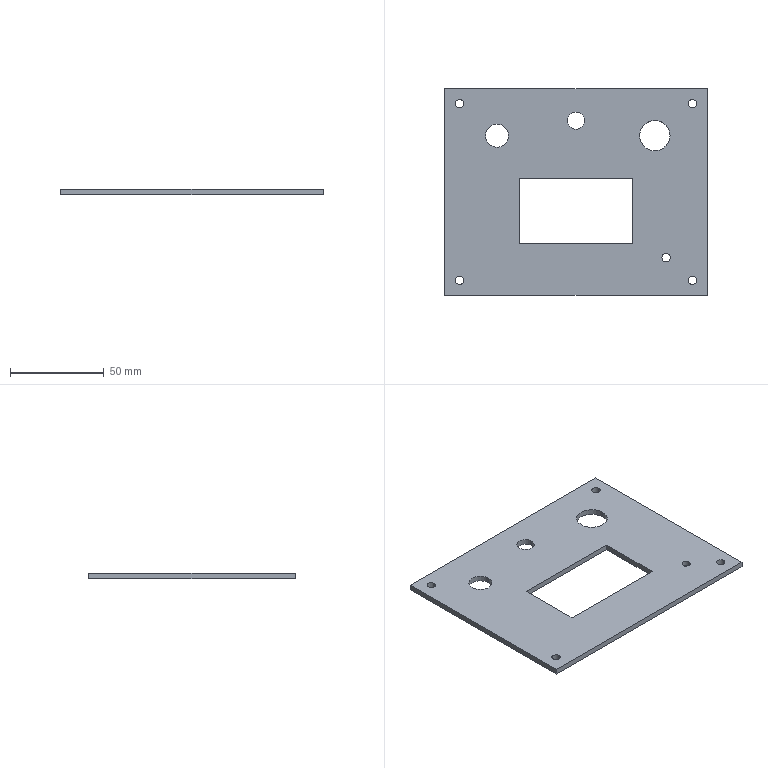Part | SolidWorks | features Extrusion 1 | 1 solid | 26 faces | box 140 x 110 x 3 mm | volume 38560 mm3 | cylinder 16 | plane 10 | commonest cylinder face diameters 4.5 x10 9.2 x2 12.2 x2 16.2 x2
STEP:
#1=CARTESIAN_POINT('',(45.75,-35.,-1.5));
#2=VERTEX_POINT('',#1);
#3=CARTESIAN_POINT('',(50.25,-35.,-1.5));
#4=VERTEX_POINT('',#3);
#5=CARTESIAN_POINT('',(48.,-35.,-1.5));
#6=DIRECTION('',(0.,0.,1.));
#7=DIRECTION('',(1.,0.,0.));
#8=AXIS2_PLACEMENT_3D('',#5,#6,#7);
#9=CIRCLE('',#8,2.25);
#10=EDGE_CURVE('',#2,#4,#9,.T.);
#11=ORIENTED_EDGE('',*,*,#10,.F.);
#12=CARTESIAN_POINT('',(45.75,-35.,1.5));
#13=VERTEX_POINT('',#12);
#14=CARTESIAN_POINT('',(45.75,-35.,-1.5));
#15=DIRECTION('',(0.,0.,1.));
#16=VECTOR('',#15,1000.);
#17=LINE('',#14,#16);
#18=EDGE_CURVE('',#2,#13,#17,.T.);
#19=ORIENTED_EDGE('',*,*,#18,.T.);
#20=CARTESIAN_POINT('',(50.25,-35.,1.5));
#21=VERTEX_POINT('',#20);
#22=CARTESIAN_POINT('',(48.,-35.,1.5));
#23=DIRECTION('',(0.,0.,1.));
#24=DIRECTION('',(1.,0.,0.));
#25=AXIS2_PLACEMENT_3D('',#22,#23,#24);
#26=CIRCLE('',#25,2.25);
#27=EDGE_CURVE('',#13,#21,#26,.T.);
#28=ORIENTED_EDGE('',*,*,#27,.T.);
#29=CARTESIAN_POINT('',(50.25,-35.,-1.5));
#30=DIRECTION('',(0.,0.,1.));
#31=VECTOR('',#30,1000.);
#32=LINE('',#29,#31);
#33=EDGE_CURVE('',#4,#21,#32,.T.);
#34=ORIENTED_EDGE('',*,*,#33,.F.);
#35=EDGE_LOOP('',(#11,#19,#28,#34));
#36=FACE_OUTER_BOUND('',#35,.T.);
#37=CARTESIAN_POINT('',(48.,-35.,-1.5));
#38=DIRECTION('',(0.,0.,1.));
#39=DIRECTION('',(1.,0.,0.));
#40=AXIS2_PLACEMENT_3D('',#37,#38,#39);
#41=CYLINDRICAL_SURFACE('',#40,2.25);
#42=ADVANCED_FACE('',(#36),#41,.F.);
#43=CARTESIAN_POINT('',(-4.6,38.,-1.5));
#44=VERTEX_POINT('',#43);
#45=CARTESIAN_POINT('',(4.6,38.,-1.5));
#46=VERTEX_POINT('',#45);
#47=CARTESIAN_POINT('',(0.,38.,-1.5));
#48=DIRECTION('',(0.,0.,1.));
#49=DIRECTION('',(1.,0.,0.));
#50=AXIS2_PLACEMENT_3D('',#47,#48,#49);
#51=CIRCLE('',#50,4.6);
#52=EDGE_CURVE('',#44,#46,#51,.T.);
#53=ORIENTED_EDGE('',*,*,#52,.F.);
#54=CARTESIAN_POINT('',(-4.6,38.,1.5));
#55=VERTEX_POINT('',#54);
#56=CARTESIAN_POINT('',(-4.6,38.,-1.5));
#57=DIRECTION('',(0.,0.,1.));
#58=VECTOR('',#57,1000.);
#59=LINE('',#56,#58);
#60=EDGE_CURVE('',#44,#55,#59,.T.);
#61=ORIENTED_EDGE('',*,*,#60,.T.);
#62=CARTESIAN_POINT('',(4.6,38.,1.5));
#63=VERTEX_POINT('',#62);
#64=CARTESIAN_POINT('',(0.,38.,1.5));
#65=DIRECTION('',(0.,0.,1.));
#66=DIRECTION('',(1.,0.,0.));
#67=AXIS2_PLACEMENT_3D('',#64,#65,#66);
#68=CIRCLE('',#67,4.6);
#69=EDGE_CURVE('',#55,#63,#68,.T.);
#70=ORIENTED_EDGE('',*,*,#69,.T.);
#71=CARTESIAN_POINT('',(4.6,38.,-1.5));
#72=DIRECTION('',(0.,0.,1.));
#73=VECTOR('',#72,1000.);
#74=LINE('',#71,#73);
#75=EDGE_CURVE('',#46,#63,#74,.T.);
#76=ORIENTED_EDGE('',*,*,#75,.F.);
#77=EDGE_LOOP('',(#53,#61,#70,#76));
#78=FACE_OUTER_BOUND('',#77,.T.);
#79=CARTESIAN_POINT('',(0.,38.,-1.5));
#80=DIRECTION('',(0.,0.,1.));
#81=DIRECTION('',(1.,0.,0.));
#82=AXIS2_PLACEMENT_3D('',#79,#80,#81);
#83=CYLINDRICAL_SURFACE('',#82,4.6);
#84=ADVANCED_FACE('',(#78),#83,.F.);
#85=CARTESIAN_POINT('',(33.9,30.,-1.5));
#86=VERTEX_POINT('',#85);
#87=CARTESIAN_POINT('',(50.1,30.,-1.5));
#88=VERTEX_POINT('',#87);
#89=CARTESIAN_POINT('',(42.,30.,-1.5));
#90=DIRECTION('',(0.,0.,1.));
#91=DIRECTION('',(1.,0.,0.));
#92=AXIS2_PLACEMENT_3D('',#89,#90,#91);
#93=CIRCLE('',#92,8.1);
#94=EDGE_CURVE('',#86,#88,#93,.T.);
#95=ORIENTED_EDGE('',*,*,#94,.F.);
#96=CARTESIAN_POINT('',(33.9,30.,1.5));
#97=VERTEX_POINT('',#96);
#98=CARTESIAN_POINT('',(33.9,30.,-1.5));
#99=DIRECTION('',(0.,0.,1.));
#100=VECTOR('',#99,1000.);
#101=LINE('',#98,#100);
#102=EDGE_CURVE('',#86,#97,#101,.T.);
#103=ORIENTED_EDGE('',*,*,#102,.T.);
#104=CARTESIAN_POINT('',(50.1,30.,1.5));
#105=VERTEX_POINT('',#104);
#106=CARTESIAN_POINT('',(42.,30.,1.5));
#107=DIRECTION('',(0.,0.,1.));
#108=DIRECTION('',(1.,0.,0.));
#109=AXIS2_PLACEMENT_3D('',#106,#107,#108);
#110=CIRCLE('',#109,8.1);
#111=EDGE_CURVE('',#97,#105,#110,.T.);
#112=ORIENTED_EDGE('',*,*,#111,.T.);
#113=CARTESIAN_POINT('',(50.1,30.,-1.5));
#114=DIRECTION('',(0.,0.,1.));
#115=VECTOR('',#114,1000.);
#116=LINE('',#113,#115);
#117=EDGE_CURVE('',#88,#105,#116,.T.);
#118=ORIENTED_EDGE('',*,*,#117,.F.);
#119=EDGE_LOOP('',(#95,#103,#112,#118));
#120=FACE_OUTER_BOUND('',#119,.T.);
#121=CARTESIAN_POINT('',(42.,30.,-1.5));
#122=DIRECTION('',(0.,0.,1.));
#123=DIRECTION('',(1.,0.,0.));
#124=AXIS2_PLACEMENT_3D('',#121,#122,#123);
#125=CYLINDRICAL_SURFACE('',#124,8.1);
#126=ADVANCED_FACE('',(#120),#125,.F.);
#127=CARTESIAN_POINT('',(-48.1,30.,-1.5));
#128=VERTEX_POINT('',#127);
#129=CARTESIAN_POINT('',(-35.9,30.,-1.5));
#130=VERTEX_POINT('',#129);
#131=CARTESIAN_POINT('',(-42.,30.,-1.5));
#132=DIRECTION('',(0.,0.,1.));
#133=DIRECTION('',(1.,0.,0.));
#134=AXIS2_PLACEMENT_3D('',#131,#132,#133);
#135=CIRCLE('',#134,6.1);
#136=EDGE_CURVE('',#128,#130,#135,.T.);
#137=ORIENTED_EDGE('',*,*,#136,.F.);
#138=CARTESIAN_POINT('',(-48.1,30.,1.5));
#139=VERTEX_POINT('',#138);
#140=CARTESIAN_POINT('',(-48.1,30.,-1.5));
#141=DIRECTION('',(0.,0.,1.));
#142=VECTOR('',#141,1000.);
#143=LINE('',#140,#142);
#144=EDGE_CURVE('',#128,#139,#143,.T.);
#145=ORIENTED_EDGE('',*,*,#144,.T.);
#146=CARTESIAN_POINT('',(-35.9,30.,1.5));
#147=VERTEX_POINT('',#146);
#148=CARTESIAN_POINT('',(-42.,30.,1.5));
#149=DIRECTION('',(0.,0.,1.));
#150=DIRECTION('',(1.,0.,0.));
#151=AXIS2_PLACEMENT_3D('',#148,#149,#150);
#152=CIRCLE('',#151,6.1);
#153=EDGE_CURVE('',#139,#147,#152,.T.);
#154=ORIENTED_EDGE('',*,*,#153,.T.);
#155=CARTESIAN_POINT('',(-35.9,30.,-1.5));
#156=DIRECTION('',(0.,0.,1.));
#157=VECTOR('',#156,1000.);
#158=LINE('',#155,#157);
#159=EDGE_CURVE('',#130,#147,#158,.T.);
#160=ORIENTED_EDGE('',*,*,#159,.F.);
#161=EDGE_LOOP('',(#137,#145,#154,#160));
#162=FACE_OUTER_BOUND('',#161,.T.);
#163=CARTESIAN_POINT('',(-42.,30.,-1.5));
#164=DIRECTION('',(0.,0.,1.));
#165=DIRECTION('',(1.,0.,0.));
#166=AXIS2_PLACEMENT_3D('',#163,#164,#165);
#167=CYLINDRICAL_SURFACE('',#166,6.1);
#168=ADVANCED_FACE('',(#162),#167,.F.);
#169=CARTESIAN_POINT('',(59.75,47.,-1.5));
#170=VERTEX_POINT('',#169);
#171=CARTESIAN_POINT('',(64.25,47.,-1.5));
#172=VERTEX_POINT('',#171);
#173=CARTESIAN_POINT('',(62.,47.,-1.5));
#174=DIRECTION('',(0.,0.,1.));
#175=DIRECTION('',(1.,0.,0.));
#176=AXIS2_PLACEMENT_3D('',#173,#174,#175);
#177=CIRCLE('',#176,2.25);
#178=EDGE_CURVE('',#170,#172,#177,.T.);
#179=ORIENTED_EDGE('',*,*,#178,.F.);
#180=CARTESIAN_POINT('',(59.75,47.,1.5));
#181=VERTEX_POINT('',#180);
#182=CARTESIAN_POINT('',(59.75,47.,-1.5));
#183=DIRECTION('',(0.,0.,1.));
#184=VECTOR('',#183,1000.);
#185=LINE('',#182,#184);
#186=EDGE_CURVE('',#170,#181,#185,.T.);
#187=ORIENTED_EDGE('',*,*,#186,.T.);
#188=CARTESIAN_POINT('',(64.25,47.,1.5));
#189=VERTEX_POINT('',#188);
#190=CARTESIAN_POINT('',(62.,47.,1.5));
#191=DIRECTION('',(0.,0.,1.));
#192=DIRECTION('',(1.,0.,0.));
#193=AXIS2_PLACEMENT_3D('',#190,#191,#192);
#194=CIRCLE('',#193,2.25);
#195=EDGE_CURVE('',#181,#189,#194,.T.);
#196=ORIENTED_EDGE('',*,*,#195,.T.);
#197=CARTESIAN_POINT('',(64.25,47.,-1.5));
#198=DIRECTION('',(0.,0.,1.));
#199=VECTOR('',#198,1000.);
#200=LINE('',#197,#199);
#201=EDGE_CURVE('',#172,#189,#200,.T.);
#202=ORIENTED_EDGE('',*,*,#201,.F.);
#203=EDGE_LOOP('',(#179,#187,#196,#202));
#204=FACE_OUTER_BOUND('',#203,.T.);
#205=CARTESIAN_POINT('',(62.,47.,-1.5));
#206=DIRECTION('',(0.,0.,1.));
#207=DIRECTION('',(1.,0.,0.));
#208=AXIS2_PLACEMENT_3D('',#205,#206,#207);
#209=CYLINDRICAL_SURFACE('',#208,2.25);
#210=ADVANCED_FACE('',(#204),#209,.F.);
#211=CARTESIAN_POINT('',(59.75,-47.,-1.5));
#212=VERTEX_POINT('',#211);
#213=CARTESIAN_POINT('',(64.25,-47.,-1.5));
#214=VERTEX_POINT('',#213);
#215=CARTESIAN_POINT('',(62.,-47.,-1.5));
#216=DIRECTION('',(0.,0.,1.));
#217=DIRECTION('',(1.,0.,0.));
#218=AXIS2_PLACEMENT_3D('',#215,#216,#217);
#219=CIRCLE('',#218,2.25);
#220=EDGE_CURVE('',#212,#214,#219,.T.);
#221=ORIENTED_EDGE('',*,*,#220,.F.);
#222=CARTESIAN_POINT('',(59.75,-47.,1.5));
#223=VERTEX_POINT('',#222);
#224=CARTESIAN_POINT('',(59.75,-47.,-1.5));
#225=DIRECTION('',(0.,0.,1.));
#226=VECTOR('',#225,1000.);
#227=LINE('',#224,#226);
#228=EDGE_CURVE('',#212,#223,#227,.T.);
#229=ORIENTED_EDGE('',*,*,#228,.T.);
#230=CARTESIAN_POINT('',(64.25,-47.,1.5));
#231=VERTEX_POINT('',#230);
#232=CARTESIAN_POINT('',(62.,-47.,1.5));
#233=DIRECTION('',(0.,0.,1.));
#234=DIRECTION('',(1.,0.,0.));
#235=AXIS2_PLACEMENT_3D('',#232,#233,#234);
#236=CIRCLE('',#235,2.25);
#237=EDGE_CURVE('',#223,#231,#236,.T.);
#238=ORIENTED_EDGE('',*,*,#237,.T.);
#239=CARTESIAN_POINT('',(64.25,-47.,-1.5));
#240=DIRECTION('',(0.,0.,1.));
#241=VECTOR('',#240,1000.);
#242=LINE('',#239,#241);
#243=EDGE_CURVE('',#214,#231,#242,.T.);
#244=ORIENTED_EDGE('',*,*,#243,.F.);
#245=EDGE_LOOP('',(#221,#229,#238,#244));
#246=FACE_OUTER_BOUND('',#245,.T.);
#247=CARTESIAN_POINT('',(62.,-47.,-1.5));
#248=DIRECTION('',(0.,0.,1.));
#249=DIRECTION('',(1.,0.,0.));
#250=AXIS2_PLACEMENT_3D('',#247,#248,#249);
#251=CYLINDRICAL_SURFACE('',#250,2.25);
#252=ADVANCED_FACE('',(#246),#251,.F.);
#253=CARTESIAN_POINT('',(-64.25,47.,-1.5));
#254=VERTEX_POINT('',#253);
#255=CARTESIAN_POINT('',(-59.75,47.,-1.5));
#256=VERTEX_POINT('',#255);
#257=CARTESIAN_POINT('',(-62.,47.,-1.5));
#258=DIRECTION('',(0.,0.,1.));
#259=DIRECTION('',(1.,0.,0.));
#260=AXIS2_PLACEMENT_3D('',#257,#258,#259);
#261=CIRCLE('',#260,2.25);
#262=EDGE_CURVE('',#254,#256,#261,.T.);
#263=ORIENTED_EDGE('',*,*,#262,.F.);
#264=CARTESIAN_POINT('',(-64.25,47.,1.5));
#265=VERTEX_POINT('',#264);
#266=CARTESIAN_POINT('',(-64.25,47.,-1.5));
#267=DIRECTION('',(0.,0.,1.));
#268=VECTOR('',#267,1000.);
#269=LINE('',#266,#268);
#270=EDGE_CURVE('',#254,#265,#269,.T.);
#271=ORIENTED_EDGE('',*,*,#270,.T.);
#272=CARTESIAN_POINT('',(-59.75,47.,1.5));
#273=VERTEX_POINT('',#272);
#274=CARTESIAN_POINT('',(-62.,47.,1.5));
#275=DIRECTION('',(0.,0.,1.));
#276=DIRECTION('',(1.,0.,0.));
#277=AXIS2_PLACEMENT_3D('',#274,#275,#276);
#278=CIRCLE('',#277,2.25);
#279=EDGE_CURVE('',#265,#273,#278,.T.);
#280=ORIENTED_EDGE('',*,*,#279,.T.);
#281=CARTESIAN_POINT('',(-59.75,47.,-1.5));
#282=DIRECTION('',(0.,0.,1.));
#283=VECTOR('',#282,1000.);
#284=LINE('',#281,#283);
#285=EDGE_CURVE('',#256,#273,#284,.T.);
#286=ORIENTED_EDGE('',*,*,#285,.F.);
#287=EDGE_LOOP('',(#263,#271,#280,#286));
#288=FACE_OUTER_BOUND('',#287,.T.);
#289=CARTESIAN_POINT('',(-62.,47.,-1.5));
#290=DIRECTION('',(0.,0.,1.));
#291=DIRECTION('',(1.,0.,0.));
#292=AXIS2_PLACEMENT_3D('',#289,#290,#291);
#293=CYLINDRICAL_SURFACE('',#292,2.25);
#294=ADVANCED_FACE('',(#288),#293,.F.);
#295=CARTESIAN_POINT('',(-64.25,-47.,-1.5));
#296=VERTEX_POINT('',#295);
#297=CARTESIAN_POINT('',(-59.75,-47.,-1.5));
#298=VERTEX_POINT('',#297);
#299=CARTESIAN_POINT('',(-62.,-47.,-1.5));
#300=DIRECTION('',(0.,0.,1.));
#301=DIRECTION('',(1.,0.,0.));
#302=AXIS2_PLACEMENT_3D('',#299,#300,#301);
#303=CIRCLE('',#302,2.25);
#304=EDGE_CURVE('',#296,#298,#303,.T.);
#305=ORIENTED_EDGE('',*,*,#304,.F.);
#306=CARTESIAN_POINT('',(-64.25,-47.,1.5));
#307=VERTEX_POINT('',#306);
#308=CARTESIAN_POINT('',(-64.25,-47.,-1.5));
#309=DIRECTION('',(0.,0.,1.));
#310=VECTOR('',#309,1000.);
#311=LINE('',#308,#310);
#312=EDGE_CURVE('',#296,#307,#311,.T.);
#313=ORIENTED_EDGE('',*,*,#312,.T.);
#314=CARTESIAN_POINT('',(-59.75,-47.,1.5));
#315=VERTEX_POINT('',#314);
#316=CARTESIAN_POINT('',(-62.,-47.,1.5));
#317=DIRECTION('',(0.,0.,1.));
#318=DIRECTION('',(1.,0.,0.));
#319=AXIS2_PLACEMENT_3D('',#316,#317,#318);
#320=CIRCLE('',#319,2.25);
#321=EDGE_CURVE('',#307,#315,#320,.T.);
#322=ORIENTED_EDGE('',*,*,#321,.T.);
#323=CARTESIAN_POINT('',(-59.75,-47.,-1.5));
#324=DIRECTION('',(0.,0.,1.));
#325=VECTOR('',#324,1000.);
#326=LINE('',#323,#325);
#327=EDGE_CURVE('',#298,#315,#326,.T.);
#328=ORIENTED_EDGE('',*,*,#327,.F.);
#329=EDGE_LOOP('',(#305,#313,#322,#328));
#330=FACE_OUTER_BOUND('',#329,.T.);
#331=CARTESIAN_POINT('',(-62.,-47.,-1.5));
#332=DIRECTION('',(0.,0.,1.));
#333=DIRECTION('',(1.,0.,0.));
#334=AXIS2_PLACEMENT_3D('',#331,#332,#333);
#335=CYLINDRICAL_SURFACE('',#334,2.25);
#336=ADVANCED_FACE('',(#330),#335,.F.);
#337=CARTESIAN_POINT('',(-70.,55.,1.5));
#338=VERTEX_POINT('',#337);
#339=CARTESIAN_POINT('',(-70.,-55.,1.5));
#340=VERTEX_POINT('',#339);
#341=CARTESIAN_POINT('',(-70.,55.,1.5));
#342=DIRECTION('',(0.,-1.,0.));
#343=VECTOR('',#342,1000.);
#344=LINE('',#341,#343);
#345=EDGE_CURVE('',#338,#340,#344,.T.);
#346=ORIENTED_EDGE('',*,*,#345,.F.);
#347=CARTESIAN_POINT('',(-70.,55.,-1.5));
#348=VERTEX_POINT('',#347);
#349=CARTESIAN_POINT('',(-70.,55.,-1.5));
#350=DIRECTION('',(0.,0.,1.));
#351=VECTOR('',#350,1000.);
#352=LINE('',#349,#351);
#353=EDGE_CURVE('',#348,#338,#352,.T.);
#354=ORIENTED_EDGE('',*,*,#353,.F.);
#355=CARTESIAN_POINT('',(-70.,-55.,-1.5));
#356=VERTEX_POINT('',#355);
#357=CARTESIAN_POINT('',(-70.,55.,-1.5));
#358=DIRECTION('',(0.,-1.,0.));
#359=VECTOR('',#358,1000.);
#360=LINE('',#357,#359);
#361=EDGE_CURVE('',#348,#356,#360,.T.);
#362=ORIENTED_EDGE('',*,*,#361,.T.);
#363=CARTESIAN_POINT('',(-70.,-55.,-1.5));
#364=DIRECTION('',(0.,0.,1.));
#365=VECTOR('',#364,1000.);
#366=LINE('',#363,#365);
#367=EDGE_CURVE('',#356,#340,#366,.T.);
#368=ORIENTED_EDGE('',*,*,#367,.T.);
#369=EDGE_LOOP('',(#346,#354,#362,#368));
#370=FACE_OUTER_BOUND('',#369,.T.);
#371=CARTESIAN_POINT('',(-70.,55.,-1.5));
#372=DIRECTION('',(-1.,0.,0.));
#373=DIRECTION('',(0.,0.,1.));
#374=AXIS2_PLACEMENT_3D('',#371,#372,#373);
#375=PLANE('',#374);
#376=ADVANCED_FACE('',(#370),#375,.T.);
#377=CARTESIAN_POINT('',(70.,55.,1.5));
#378=VERTEX_POINT('',#377);
#379=CARTESIAN_POINT('',(70.,55.,1.5));
#380=DIRECTION('',(-1.,0.,0.));
#381=VECTOR('',#380,1000.);
#382=LINE('',#379,#381);
#383=EDGE_CURVE('',#378,#338,#382,.T.);
#384=ORIENTED_EDGE('',*,*,#383,.F.);
#385=CARTESIAN_POINT('',(70.,55.,-1.5));
#386=VERTEX_POINT('',#385);
#387=CARTESIAN_POINT('',(70.,55.,-1.5));
#388=DIRECTION('',(0.,0.,1.));
#389=VECTOR('',#388,1000.);
#390=LINE('',#387,#389);
#391=EDGE_CURVE('',#386,#378,#390,.T.);
#392=ORIENTED_EDGE('',*,*,#391,.F.);
#393=CARTESIAN_POINT('',(70.,55.,-1.5));
#394=DIRECTION('',(-1.,0.,0.));
#395=VECTOR('',#394,1000.);
#396=LINE('',#393,#395);
#397=EDGE_CURVE('',#386,#348,#396,.T.);
#398=ORIENTED_EDGE('',*,*,#397,.T.);
#399=ORIENTED_EDGE('',*,*,#353,.T.);
#400=EDGE_LOOP('',(#384,#392,#398,#399));
#401=FACE_OUTER_BOUND('',#400,.T.);
#402=CARTESIAN_POINT('',(70.,55.,-1.5));
#403=DIRECTION('',(0.,1.,0.));
#404=DIRECTION('',(0.,0.,1.));
#405=AXIS2_PLACEMENT_3D('',#402,#403,#404);
#406=PLANE('',#405);
#407=ADVANCED_FACE('',(#401),#406,.T.);
#408=CARTESIAN_POINT('',(70.,-55.,1.5));
#409=VERTEX_POINT('',#408);
#410=CARTESIAN_POINT('',(70.,-55.,1.5));
#411=DIRECTION('',(0.,1.,0.));
#412=VECTOR('',#411,1000.);
#413=LINE('',#410,#412);
#414=EDGE_CURVE('',#409,#378,#413,.T.);
#415=ORIENTED_EDGE('',*,*,#414,.F.);
#416=CARTESIAN_POINT('',(70.,-55.,-1.5));
#417=VERTEX_POINT('',#416);
#418=CARTESIAN_POINT('',(70.,-55.,-1.5));
#419=DIRECTION('',(0.,0.,1.));
#420=VECTOR('',#419,1000.);
#421=LINE('',#418,#420);
#422=EDGE_CURVE('',#417,#409,#421,.T.);
#423=ORIENTED_EDGE('',*,*,#422,.F.);
#424=CARTESIAN_POINT('',(70.,-55.,-1.5));
#425=DIRECTION('',(0.,1.,0.));
#426=VECTOR('',#425,1000.);
#427=LINE('',#424,#426);
#428=EDGE_CURVE('',#417,#386,#427,.T.);
#429=ORIENTED_EDGE('',*,*,#428,.T.);
#430=ORIENTED_EDGE('',*,*,#391,.T.);
#431=EDGE_LOOP('',(#415,#423,#429,#430));
#432=FACE_OUTER_BOUND('',#431,.T.);
#433=CARTESIAN_POINT('',(70.,-55.,-1.5));
#434=DIRECTION('',(1.,0.,0.));
#435=DIRECTION('',(0.,0.,-1.));
#436=AXIS2_PLACEMENT_3D('',#433,#434,#435);
#437=PLANE('',#436);
#438=ADVANCED_FACE('',(#432),#437,.T.);
#439=CARTESIAN_POINT('',(-70.,-55.,1.5));
#440=DIRECTION('',(1.,0.,0.));
#441=VECTOR('',#440,1000.);
#442=LINE('',#439,#441);
#443=EDGE_CURVE('',#340,#409,#442,.T.);
#444=ORIENTED_EDGE('',*,*,#443,.F.);
#445=ORIENTED_EDGE('',*,*,#367,.F.);
#446=CARTESIAN_POINT('',(-70.,-55.,-1.5));
#447=DIRECTION('',(1.,0.,0.));
#448=VECTOR('',#447,1000.);
#449=LINE('',#446,#448);
#450=EDGE_CURVE('',#356,#417,#449,.T.);
#451=ORIENTED_EDGE('',*,*,#450,.T.);
#452=ORIENTED_EDGE('',*,*,#422,.T.);
#453=EDGE_LOOP('',(#444,#445,#451,#452));
#454=FACE_OUTER_BOUND('',#453,.T.);
#455=CARTESIAN_POINT('',(-70.,-55.,-1.5));
#456=DIRECTION('',(0.,-1.,0.));
#457=DIRECTION('',(0.,0.,-1.));
#458=AXIS2_PLACEMENT_3D('',#455,#456,#457);
#459=PLANE('',#458);
#460=ADVANCED_FACE('',(#454),#459,.T.);
#461=CARTESIAN_POINT('',(48.,-35.,-1.5));
#462=DIRECTION('',(0.,0.,1.));
#463=DIRECTION('',(1.,0.,0.));
#464=AXIS2_PLACEMENT_3D('',#461,#462,#463);
#465=CIRCLE('',#464,2.25);
#466=EDGE_CURVE('',#4,#2,#465,.T.);
#467=ORIENTED_EDGE('',*,*,#466,.T.);
#468=ORIENTED_EDGE('',*,*,#10,.T.);
#469=EDGE_LOOP('',(#467,#468));
#470=FACE_BOUND('',#469,.T.);
#471=CARTESIAN_POINT('',(0.,38.,-1.5));
#472=DIRECTION('',(0.,0.,1.));
#473=DIRECTION('',(1.,0.,0.));
#474=AXIS2_PLACEMENT_3D('',#471,#472,#473);
#475=CIRCLE('',#474,4.6);
#476=EDGE_CURVE('',#46,#44,#475,.T.);
#477=ORIENTED_EDGE('',*,*,#476,.T.);
#478=ORIENTED_EDGE('',*,*,#52,.T.);
#479=EDGE_LOOP('',(#477,#478));
#480=FACE_BOUND('',#479,.T.);
#481=CARTESIAN_POINT('',(42.,30.,-1.5));
#482=DIRECTION('',(0.,0.,1.));
#483=DIRECTION('',(1.,0.,0.));
#484=AXIS2_PLACEMENT_3D('',#481,#482,#483);
#485=CIRCLE('',#484,8.1);
#486=EDGE_CURVE('',#88,#86,#485,.T.);
#487=ORIENTED_EDGE('',*,*,#486,.T.);
#488=ORIENTED_EDGE('',*,*,#94,.T.);
#489=EDGE_LOOP('',(#487,#488));
#490=FACE_BOUND('',#489,.T.);
#491=CARTESIAN_POINT('',(-42.,30.,-1.5));
#492=DIRECTION('',(0.,0.,1.));
#493=DIRECTION('',(1.,0.,0.));
#494=AXIS2_PLACEMENT_3D('',#491,#492,#493);
#495=CIRCLE('',#494,6.1);
#496=EDGE_CURVE('',#130,#128,#495,.T.);
#497=ORIENTED_EDGE('',*,*,#496,.T.);
#498=ORIENTED_EDGE('',*,*,#136,.T.);
#499=EDGE_LOOP('',(#497,#498));
#500=FACE_BOUND('',#499,.T.);
#501=CARTESIAN_POINT('',(62.,47.,-1.5));
#502=DIRECTION('',(0.,0.,1.));
#503=DIRECTION('',(1.,0.,0.));
#504=AXIS2_PLACEMENT_3D('',#501,#502,#503);
#505=CIRCLE('',#504,2.25);
#506=EDGE_CURVE('',#172,#170,#505,.T.);
#507=ORIENTED_EDGE('',*,*,#506,.T.);
#508=ORIENTED_EDGE('',*,*,#178,.T.);
#509=EDGE_LOOP('',(#507,#508));
#510=FACE_BOUND('',#509,.T.);
#511=CARTESIAN_POINT('',(62.,-47.,-1.5));
#512=DIRECTION('',(0.,0.,1.));
#513=DIRECTION('',(1.,0.,0.));
#514=AXIS2_PLACEMENT_3D('',#511,#512,#513);
#515=CIRCLE('',#514,2.25);
#516=EDGE_CURVE('',#214,#212,#515,.T.);
#517=ORIENTED_EDGE('',*,*,#516,.T.);
#518=ORIENTED_EDGE('',*,*,#220,.T.);
#519=EDGE_LOOP('',(#517,#518));
#520=FACE_BOUND('',#519,.T.);
#521=CARTESIAN_POINT('',(-62.,47.,-1.5));
#522=DIRECTION('',(0.,0.,1.));
#523=DIRECTION('',(1.,0.,0.));
#524=AXIS2_PLACEMENT_3D('',#521,#522,#523);
#525=CIRCLE('',#524,2.25);
#526=EDGE_CURVE('',#256,#254,#525,.T.);
#527=ORIENTED_EDGE('',*,*,#526,.T.);
#528=ORIENTED_EDGE('',*,*,#262,.T.);
#529=EDGE_LOOP('',(#527,#528));
#530=FACE_BOUND('',#529,.T.);
#531=CARTESIAN_POINT('',(-62.,-47.,-1.5));
#532=DIRECTION('',(0.,0.,1.));
#533=DIRECTION('',(1.,0.,0.));
#534=AXIS2_PLACEMENT_3D('',#531,#532,#533);
#535=CIRCLE('',#534,2.25);
#536=EDGE_CURVE('',#298,#296,#535,.T.);
#537=ORIENTED_EDGE('',*,*,#536,.T.);
#538=ORIENTED_EDGE('',*,*,#304,.T.);
#539=EDGE_LOOP('',(#537,#538));
#540=FACE_BOUND('',#539,.T.);
#541=CARTESIAN_POINT('',(30.2,7.2,-1.5));
#542=VERTEX_POINT('',#541);
#543=CARTESIAN_POINT('',(-30.2,7.2,-1.5));
#544=VERTEX_POINT('',#543);
#545=CARTESIAN_POINT('',(30.2,7.2,-1.5));
#546=DIRECTION('',(-1.,0.,0.));
#547=VECTOR('',#546,1000.);
#548=LINE('',#545,#547);
#549=EDGE_CURVE('',#542,#544,#548,.T.);
#550=ORIENTED_EDGE('',*,*,#549,.T.);
#551=CARTESIAN_POINT('',(-30.2,-27.2,-1.5));
#552=VERTEX_POINT('',#551);
#553=CARTESIAN_POINT('',(-30.2,7.2,-1.5));
#554=DIRECTION('',(0.,-1.,0.));
#555=VECTOR('',#554,1000.);
#556=LINE('',#553,#555);
#557=EDGE_CURVE('',#544,#552,#556,.T.);
#558=ORIENTED_EDGE('',*,*,#557,.T.);
#559=CARTESIAN_POINT('',(30.2,-27.2,-1.5));
#560=VERTEX_POINT('',#559);
#561=CARTESIAN_POINT('',(-30.2,-27.2,-1.5));
#562=DIRECTION('',(1.,0.,0.));
#563=VECTOR('',#562,1000.);
#564=LINE('',#561,#563);
#565=EDGE_CURVE('',#552,#560,#564,.T.);
#566=ORIENTED_EDGE('',*,*,#565,.T.);
#567=CARTESIAN_POINT('',(30.2,-27.2,-1.5));
#568=DIRECTION('',(0.,1.,0.));
#569=VECTOR('',#568,1000.);
#570=LINE('',#567,#569);
#571=EDGE_CURVE('',#560,#542,#570,.T.);
#572=ORIENTED_EDGE('',*,*,#571,.T.);
#573=EDGE_LOOP('',(#550,#558,#566,#572));
#574=FACE_BOUND('',#573,.T.);
#575=ORIENTED_EDGE('',*,*,#361,.F.);
#576=ORIENTED_EDGE('',*,*,#397,.F.);
#577=ORIENTED_EDGE('',*,*,#428,.F.);
#578=ORIENTED_EDGE('',*,*,#450,.F.);
#579=EDGE_LOOP('',(#575,#576,#577,#578));
#580=FACE_OUTER_BOUND('',#579,.T.);
#581=CARTESIAN_POINT('',(0.,0.,-1.5));
#582=DIRECTION('',(0.,0.,1.));
#583=DIRECTION('',(1.,0.,0.));
#584=AXIS2_PLACEMENT_3D('',#581,#582,#583);
#585=PLANE('',#584);
#586=ADVANCED_FACE('',(#470,#480,#490,#500,#510,#520,#530,#540,#574,#580),#585,.F.);
#587=CARTESIAN_POINT('',(48.,-35.,1.5));
#588=DIRECTION('',(0.,0.,1.));
#589=DIRECTION('',(1.,0.,0.));
#590=AXIS2_PLACEMENT_3D('',#587,#588,#589);
#591=CIRCLE('',#590,2.25);
#592=EDGE_CURVE('',#21,#13,#591,.T.);
#593=ORIENTED_EDGE('',*,*,#592,.F.);
#594=ORIENTED_EDGE('',*,*,#27,.F.);
#595=EDGE_LOOP('',(#593,#594));
#596=FACE_BOUND('',#595,.T.);
#597=CARTESIAN_POINT('',(0.,38.,1.5));
#598=DIRECTION('',(0.,0.,1.));
#599=DIRECTION('',(1.,0.,0.));
#600=AXIS2_PLACEMENT_3D('',#597,#598,#599);
#601=CIRCLE('',#600,4.6);
#602=EDGE_CURVE('',#63,#55,#601,.T.);
#603=ORIENTED_EDGE('',*,*,#602,.F.);
#604=ORIENTED_EDGE('',*,*,#69,.F.);
#605=EDGE_LOOP('',(#603,#604));
#606=FACE_BOUND('',#605,.T.);
#607=CARTESIAN_POINT('',(42.,30.,1.5));
#608=DIRECTION('',(0.,0.,1.));
#609=DIRECTION('',(1.,0.,0.));
#610=AXIS2_PLACEMENT_3D('',#607,#608,#609);
#611=CIRCLE('',#610,8.1);
#612=EDGE_CURVE('',#105,#97,#611,.T.);
#613=ORIENTED_EDGE('',*,*,#612,.F.);
#614=ORIENTED_EDGE('',*,*,#111,.F.);
#615=EDGE_LOOP('',(#613,#614));
#616=FACE_BOUND('',#615,.T.);
#617=CARTESIAN_POINT('',(-42.,30.,1.5));
#618=DIRECTION('',(0.,0.,1.));
#619=DIRECTION('',(1.,0.,0.));
#620=AXIS2_PLACEMENT_3D('',#617,#618,#619);
#621=CIRCLE('',#620,6.1);
#622=EDGE_CURVE('',#147,#139,#621,.T.);
#623=ORIENTED_EDGE('',*,*,#622,.F.);
#624=ORIENTED_EDGE('',*,*,#153,.F.);
#625=EDGE_LOOP('',(#623,#624));
#626=FACE_BOUND('',#625,.T.);
#627=CARTESIAN_POINT('',(62.,47.,1.5));
#628=DIRECTION('',(0.,0.,1.));
#629=DIRECTION('',(1.,0.,0.));
#630=AXIS2_PLACEMENT_3D('',#627,#628,#629);
#631=CIRCLE('',#630,2.25);
#632=EDGE_CURVE('',#189,#181,#631,.T.);
#633=ORIENTED_EDGE('',*,*,#632,.F.);
#634=ORIENTED_EDGE('',*,*,#195,.F.);
#635=EDGE_LOOP('',(#633,#634));
#636=FACE_BOUND('',#635,.T.);
#637=CARTESIAN_POINT('',(62.,-47.,1.5));
#638=DIRECTION('',(0.,0.,1.));
#639=DIRECTION('',(1.,0.,0.));
#640=AXIS2_PLACEMENT_3D('',#637,#638,#639);
#641=CIRCLE('',#640,2.25);
#642=EDGE_CURVE('',#231,#223,#641,.T.);
#643=ORIENTED_EDGE('',*,*,#642,.F.);
#644=ORIENTED_EDGE('',*,*,#237,.F.);
#645=EDGE_LOOP('',(#643,#644));
#646=FACE_BOUND('',#645,.T.);
#647=CARTESIAN_POINT('',(-62.,47.,1.5));
#648=DIRECTION('',(0.,0.,1.));
#649=DIRECTION('',(1.,0.,0.));
#650=AXIS2_PLACEMENT_3D('',#647,#648,#649);
#651=CIRCLE('',#650,2.25);
#652=EDGE_CURVE('',#273,#265,#651,.T.);
#653=ORIENTED_EDGE('',*,*,#652,.F.);
#654=ORIENTED_EDGE('',*,*,#279,.F.);
#655=EDGE_LOOP('',(#653,#654));
#656=FACE_BOUND('',#655,.T.);
#657=CARTESIAN_POINT('',(-62.,-47.,1.5));
#658=DIRECTION('',(0.,0.,1.));
#659=DIRECTION('',(1.,0.,0.));
#660=AXIS2_PLACEMENT_3D('',#657,#658,#659);
#661=CIRCLE('',#660,2.25);
#662=EDGE_CURVE('',#315,#307,#661,.T.);
#663=ORIENTED_EDGE('',*,*,#662,.F.);
#664=ORIENTED_EDGE('',*,*,#321,.F.);
#665=EDGE_LOOP('',(#663,#664));
#666=FACE_BOUND('',#665,.T.);
#667=CARTESIAN_POINT('',(-30.2,7.2,1.5));
#668=VERTEX_POINT('',#667);
#669=CARTESIAN_POINT('',(-30.2,-27.2,1.5));
#670=VERTEX_POINT('',#669);
#671=CARTESIAN_POINT('',(-30.2,7.2,1.5));
#672=DIRECTION('',(0.,-1.,0.));
#673=VECTOR('',#672,1000.);
#674=LINE('',#671,#673);
#675=EDGE_CURVE('',#668,#670,#674,.T.);
#676=ORIENTED_EDGE('',*,*,#675,.F.);
#677=CARTESIAN_POINT('',(30.2,7.2,1.5));
#678=VERTEX_POINT('',#677);
#679=CARTESIAN_POINT('',(30.2,7.2,1.5));
#680=DIRECTION('',(-1.,0.,0.));
#681=VECTOR('',#680,1000.);
#682=LINE('',#679,#681);
#683=EDGE_CURVE('',#678,#668,#682,.T.);
#684=ORIENTED_EDGE('',*,*,#683,.F.);
#685=CARTESIAN_POINT('',(30.2,-27.2,1.5));
#686=VERTEX_POINT('',#685);
#687=CARTESIAN_POINT('',(30.2,-27.2,1.5));
#688=DIRECTION('',(0.,1.,0.));
#689=VECTOR('',#688,1000.);
#690=LINE('',#687,#689);
#691=EDGE_CURVE('',#686,#678,#690,.T.);
#692=ORIENTED_EDGE('',*,*,#691,.F.);
#693=CARTESIAN_POINT('',(-30.2,-27.2,1.5));
#694=DIRECTION('',(1.,0.,0.));
#695=VECTOR('',#694,1000.);
#696=LINE('',#693,#695);
#697=EDGE_CURVE('',#670,#686,#696,.T.);
#698=ORIENTED_EDGE('',*,*,#697,.F.);
#699=EDGE_LOOP('',(#676,#684,#692,#698));
#700=FACE_BOUND('',#699,.T.);
#701=ORIENTED_EDGE('',*,*,#345,.T.);
#702=ORIENTED_EDGE('',*,*,#443,.T.);
#703=ORIENTED_EDGE('',*,*,#414,.T.);
#704=ORIENTED_EDGE('',*,*,#383,.T.);
#705=EDGE_LOOP('',(#701,#702,#703,#704));
#706=FACE_OUTER_BOUND('',#705,.T.);
#707=CARTESIAN_POINT('',(0.,0.,1.5));
#708=DIRECTION('',(0.,0.,1.));
#709=DIRECTION('',(1.,0.,0.));
#710=AXIS2_PLACEMENT_3D('',#707,#708,#709);
#711=PLANE('',#710);
#712=ADVANCED_FACE('',(#596,#606,#616,#626,#636,#646,#656,#666,#700,#706),#711,.T.);
#713=ORIENTED_EDGE('',*,*,#675,.T.);
#714=CARTESIAN_POINT('',(-30.2,-27.2,-1.5));
#715=DIRECTION('',(0.,0.,1.));
#716=VECTOR('',#715,1000.);
#717=LINE('',#714,#716);
#718=EDGE_CURVE('',#552,#670,#717,.T.);
#719=ORIENTED_EDGE('',*,*,#718,.F.);
#720=ORIENTED_EDGE('',*,*,#557,.F.);
#721=CARTESIAN_POINT('',(-30.2,7.2,-1.5));
#722=DIRECTION('',(0.,0.,1.));
#723=VECTOR('',#722,1000.);
#724=LINE('',#721,#723);
#725=EDGE_CURVE('',#544,#668,#724,.T.);
#726=ORIENTED_EDGE('',*,*,#725,.T.);
#727=EDGE_LOOP('',(#713,#719,#720,#726));
#728=FACE_OUTER_BOUND('',#727,.T.);
#729=CARTESIAN_POINT('',(-30.2,7.2,-1.5));
#730=DIRECTION('',(-1.,0.,0.));
#731=DIRECTION('',(0.,0.,1.));
#732=AXIS2_PLACEMENT_3D('',#729,#730,#731);
#733=PLANE('',#732);
#734=ADVANCED_FACE('',(#728),#733,.F.);
#735=ORIENTED_EDGE('',*,*,#683,.T.);
#736=ORIENTED_EDGE('',*,*,#725,.F.);
#737=ORIENTED_EDGE('',*,*,#549,.F.);
#738=CARTESIAN_POINT('',(30.2,7.2,-1.5));
#739=DIRECTION('',(0.,0.,1.));
#740=VECTOR('',#739,1000.);
#741=LINE('',#738,#740);
#742=EDGE_CURVE('',#542,#678,#741,.T.);
#743=ORIENTED_EDGE('',*,*,#742,.T.);
#744=EDGE_LOOP('',(#735,#736,#737,#743));
#745=FACE_OUTER_BOUND('',#744,.T.);
#746=CARTESIAN_POINT('',(30.2,7.2,-1.5));
#747=DIRECTION('',(0.,1.,0.));
#748=DIRECTION('',(0.,0.,1.));
#749=AXIS2_PLACEMENT_3D('',#746,#747,#748);
#750=PLANE('',#749);
#751=ADVANCED_FACE('',(#745),#750,.F.);
#752=ORIENTED_EDGE('',*,*,#691,.T.);
#753=ORIENTED_EDGE('',*,*,#742,.F.);
#754=ORIENTED_EDGE('',*,*,#571,.F.);
#755=CARTESIAN_POINT('',(30.2,-27.2,-1.5));
#756=DIRECTION('',(0.,0.,1.));
#757=VECTOR('',#756,1000.);
#758=LINE('',#755,#757);
#759=EDGE_CURVE('',#560,#686,#758,.T.);
#760=ORIENTED_EDGE('',*,*,#759,.T.);
#761=EDGE_LOOP('',(#752,#753,#754,#760));
#762=FACE_OUTER_BOUND('',#761,.T.);
#763=CARTESIAN_POINT('',(30.2,-27.2,-1.5));
#764=DIRECTION('',(1.,0.,0.));
#765=DIRECTION('',(0.,0.,-1.));
#766=AXIS2_PLACEMENT_3D('',#763,#764,#765);
#767=PLANE('',#766);
#768=ADVANCED_FACE('',(#762),#767,.F.);
#769=ORIENTED_EDGE('',*,*,#697,.T.);
#770=ORIENTED_EDGE('',*,*,#759,.F.);
#771=ORIENTED_EDGE('',*,*,#565,.F.);
#772=ORIENTED_EDGE('',*,*,#718,.T.);
#773=EDGE_LOOP('',(#769,#770,#771,#772));
#774=FACE_OUTER_BOUND('',#773,.T.);
#775=CARTESIAN_POINT('',(-30.2,-27.2,-1.5));
#776=DIRECTION('',(0.,-1.,0.));
#777=DIRECTION('',(0.,0.,-1.));
#778=AXIS2_PLACEMENT_3D('',#775,#776,#777);
#779=PLANE('',#778);
#780=ADVANCED_FACE('',(#774),#779,.F.);
#781=ORIENTED_EDGE('',*,*,#312,.F.);
#782=ORIENTED_EDGE('',*,*,#536,.F.);
#783=ORIENTED_EDGE('',*,*,#327,.T.);
#784=ORIENTED_EDGE('',*,*,#662,.T.);
#785=EDGE_LOOP('',(#781,#782,#783,#784));
#786=FACE_OUTER_BOUND('',#785,.T.);
#787=CARTESIAN_POINT('',(-62.,-47.,-1.5));
#788=DIRECTION('',(0.,0.,1.));
#789=DIRECTION('',(1.,0.,0.));
#790=AXIS2_PLACEMENT_3D('',#787,#788,#789);
#791=CYLINDRICAL_SURFACE('',#790,2.25);
#792=ADVANCED_FACE('',(#786),#791,.F.);
#793=ORIENTED_EDGE('',*,*,#270,.F.);
#794=ORIENTED_EDGE('',*,*,#526,.F.);
#795=ORIENTED_EDGE('',*,*,#285,.T.);
#796=ORIENTED_EDGE('',*,*,#652,.T.);
#797=EDGE_LOOP('',(#793,#794,#795,#796));
#798=FACE_OUTER_BOUND('',#797,.T.);
#799=CARTESIAN_POINT('',(-62.,47.,-1.5));
#800=DIRECTION('',(0.,0.,1.));
#801=DIRECTION('',(1.,0.,0.));
#802=AXIS2_PLACEMENT_3D('',#799,#800,#801);
#803=CYLINDRICAL_SURFACE('',#802,2.25);
#804=ADVANCED_FACE('',(#798),#803,.F.);
#805=ORIENTED_EDGE('',*,*,#228,.F.);
#806=ORIENTED_EDGE('',*,*,#516,.F.);
#807=ORIENTED_EDGE('',*,*,#243,.T.);
#808=ORIENTED_EDGE('',*,*,#642,.T.);
#809=EDGE_LOOP('',(#805,#806,#807,#808));
#810=FACE_OUTER_BOUND('',#809,.T.);
#811=CARTESIAN_POINT('',(62.,-47.,-1.5));
#812=DIRECTION('',(0.,0.,1.));
#813=DIRECTION('',(1.,0.,0.));
#814=AXIS2_PLACEMENT_3D('',#811,#812,#813);
#815=CYLINDRICAL_SURFACE('',#814,2.25);
#816=ADVANCED_FACE('',(#810),#815,.F.);
#817=ORIENTED_EDGE('',*,*,#186,.F.);
#818=ORIENTED_EDGE('',*,*,#506,.F.);
#819=ORIENTED_EDGE('',*,*,#201,.T.);
#820=ORIENTED_EDGE('',*,*,#632,.T.);
#821=EDGE_LOOP('',(#817,#818,#819,#820));
#822=FACE_OUTER_BOUND('',#821,.T.);
#823=CARTESIAN_POINT('',(62.,47.,-1.5));
#824=DIRECTION('',(0.,0.,1.));
#825=DIRECTION('',(1.,0.,0.));
#826=AXIS2_PLACEMENT_3D('',#823,#824,#825);
#827=CYLINDRICAL_SURFACE('',#826,2.25);
#828=ADVANCED_FACE('',(#822),#827,.F.);
#829=ORIENTED_EDGE('',*,*,#144,.F.);
#830=ORIENTED_EDGE('',*,*,#496,.F.);
#831=ORIENTED_EDGE('',*,*,#159,.T.);
#832=ORIENTED_EDGE('',*,*,#622,.T.);
#833=EDGE_LOOP('',(#829,#830,#831,#832));
#834=FACE_OUTER_BOUND('',#833,.T.);
#835=CARTESIAN_POINT('',(-42.,30.,-1.5));
#836=DIRECTION('',(0.,0.,1.));
#837=DIRECTION('',(1.,0.,0.));
#838=AXIS2_PLACEMENT_3D('',#835,#836,#837);
#839=CYLINDRICAL_SURFACE('',#838,6.1);
#840=ADVANCED_FACE('',(#834),#839,.F.);
#841=ORIENTED_EDGE('',*,*,#102,.F.);
#842=ORIENTED_EDGE('',*,*,#486,.F.);
#843=ORIENTED_EDGE('',*,*,#117,.T.);
#844=ORIENTED_EDGE('',*,*,#612,.T.);
#845=EDGE_LOOP('',(#841,#842,#843,#844));
#846=FACE_OUTER_BOUND('',#845,.T.);
#847=CARTESIAN_POINT('',(42.,30.,-1.5));
#848=DIRECTION('',(0.,0.,1.));
#849=DIRECTION('',(1.,0.,0.));
#850=AXIS2_PLACEMENT_3D('',#847,#848,#849);
#851=CYLINDRICAL_SURFACE('',#850,8.1);
#852=ADVANCED_FACE('',(#846),#851,.F.);
#853=ORIENTED_EDGE('',*,*,#60,.F.);
#854=ORIENTED_EDGE('',*,*,#476,.F.);
#855=ORIENTED_EDGE('',*,*,#75,.T.);
#856=ORIENTED_EDGE('',*,*,#602,.T.);
#857=EDGE_LOOP('',(#853,#854,#855,#856));
#858=FACE_OUTER_BOUND('',#857,.T.);
#859=CARTESIAN_POINT('',(0.,38.,-1.5));
#860=DIRECTION('',(0.,0.,1.));
#861=DIRECTION('',(1.,0.,0.));
#862=AXIS2_PLACEMENT_3D('',#859,#860,#861);
#863=CYLINDRICAL_SURFACE('',#862,4.6);
#864=ADVANCED_FACE('',(#858),#863,.F.);
#865=ORIENTED_EDGE('',*,*,#18,.F.);
#866=ORIENTED_EDGE('',*,*,#466,.F.);
#867=ORIENTED_EDGE('',*,*,#33,.T.);
#868=ORIENTED_EDGE('',*,*,#592,.T.);
#869=EDGE_LOOP('',(#865,#866,#867,#868));
#870=FACE_OUTER_BOUND('',#869,.T.);
#871=CARTESIAN_POINT('',(48.,-35.,-1.5));
#872=DIRECTION('',(0.,0.,1.));
#873=DIRECTION('',(1.,0.,0.));
#874=AXIS2_PLACEMENT_3D('',#871,#872,#873);
#875=CYLINDRICAL_SURFACE('',#874,2.25);
#876=ADVANCED_FACE('',(#870),#875,.F.);
#877=CLOSED_SHELL('',(#42,#84,#126,#168,#210,#252,#294,#336,#376,#407,#438,#460,#586,#712,#734,#751,#768,#780,#792,#804,#816,#828,#840,#852,#864,#876));
#878=MANIFOLD_SOLID_BREP('',#877);
#879=CARTESIAN_POINT('',(0.,0.,0.));
#880=DIRECTION('',(0.,0.,1.));
#881=DIRECTION('',(1.,0.,0.));
#882=AXIS2_PLACEMENT_3D('',#879,#880,#881);
#883=(LENGTH_UNIT()NAMED_UNIT(*)SI_UNIT(.MILLI.,.METRE.));
#884=UNCERTAINTY_MEASURE_WITH_UNIT(LENGTH_MEASURE(0.00001),#883,'','');
#885=(NAMED_UNIT(*)PLANE_ANGLE_UNIT()SI_UNIT($,.RADIAN.));
#886=(NAMED_UNIT(*)SI_UNIT($,.STERADIAN.)SOLID_ANGLE_UNIT());
#887=(GEOMETRIC_REPRESENTATION_CONTEXT(3)GLOBAL_UNCERTAINTY_ASSIGNED_CONTEXT((#884))GLOBAL_UNIT_ASSIGNED_CONTEXT((#883,#885,#886))REPRESENTATION_CONTEXT('',''));
#888=ADVANCED_BREP_SHAPE_REPRESENTATION('',(#878,#882),#887);